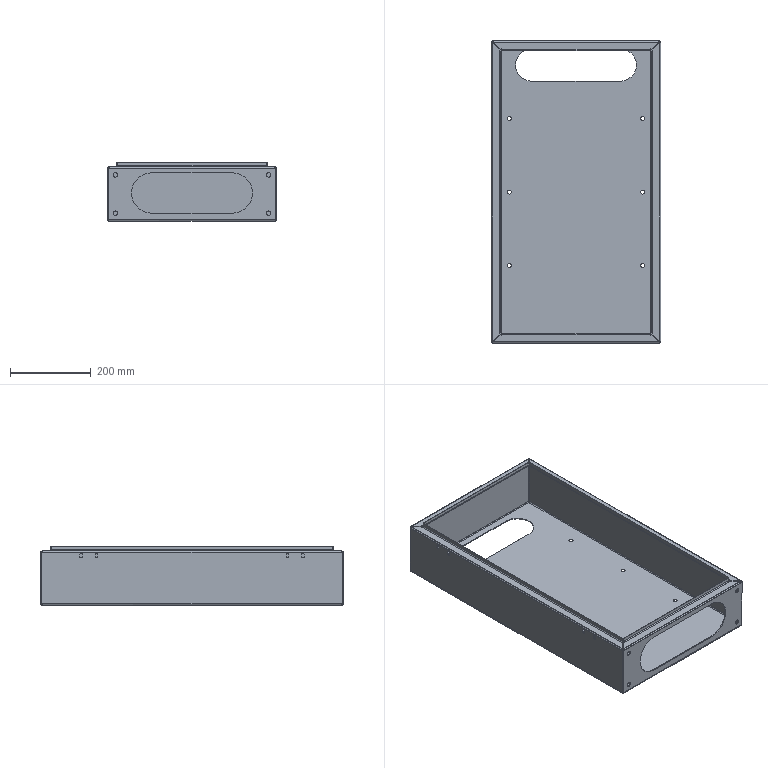Part | SolidWorks | features ICE 5, EdgeFlange 3, FlatPattern 1, SMBaseFlange 1, SheetMetal 1 | 1 solid | 175 faces | box 420 x 750 x 145 mm | volume 1270936 mm3 | plane 98 | cylinder 61 | spline 16 | commonest cylinder face diameters 4 x12 7 x12 8 x12 10 x12 11 x8 80 x3